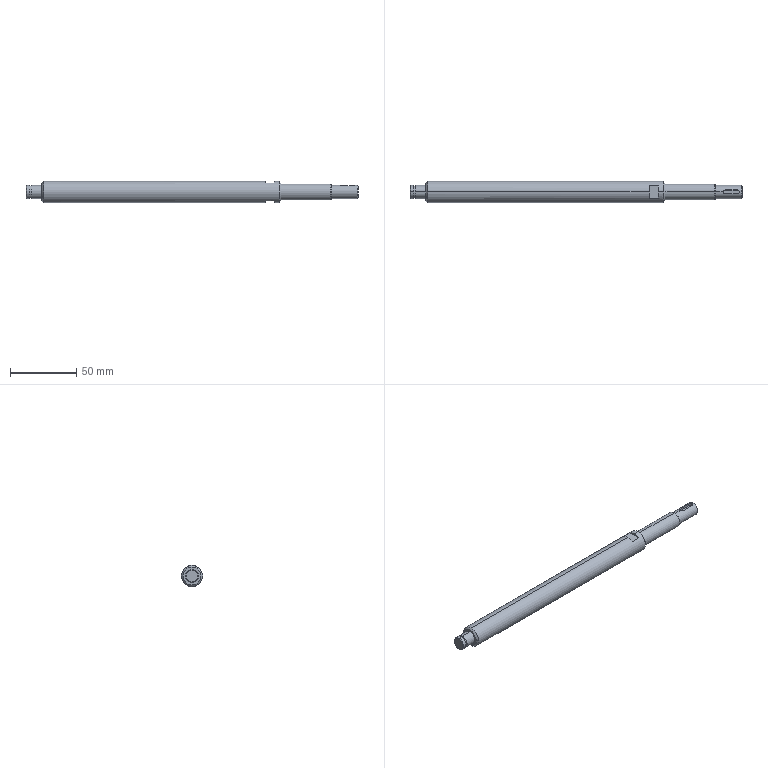Part | SolidWorks | features BaseBody 1 | 1 solid | 41 faces | box 250 x 16 x 16 mm | volume 42719 mm3 | plane 16 | cylinder 15 | cone 10 | commonest cylinder face diameters 10 x6 3 x3 9.6 x2 12 x2 16 x2
STEP:
#1=CARTESIAN_POINT('',(190.773,8.,0.));
#2=VERTEX_POINT('',#1);
#3=CARTESIAN_POINT('',(190.773,0.,-8.));
#4=VERTEX_POINT('',#3);
#5=CARTESIAN_POINT('',(190.773,0.,0.));
#6=DIRECTION('',(-1.,0.,0.));
#7=DIRECTION('',(0.,0.,1.));
#8=AXIS2_PLACEMENT_3D('',#5,#6,#7);
#9=CIRCLE('',#8,8.);
#10=EDGE_CURVE('',#2,#4,#9,.T.);
#11=ORIENTED_EDGE('',*,*,#10,.T.);
#12=CARTESIAN_POINT('',(187.,0.,-8.));
#13=VERTEX_POINT('',#12);
#14=CARTESIAN_POINT('',(250.,0.,-8.));
#15=DIRECTION('',(-1.,0.,0.));
#16=VECTOR('',#15,1000.);
#17=LINE('',#14,#16);
#18=EDGE_CURVE('',#4,#13,#17,.T.);
#19=ORIENTED_EDGE('',*,*,#18,.T.);
#20=CARTESIAN_POINT('',(187.,4.664,-6.5));
#21=VERTEX_POINT('',#20);
#22=CARTESIAN_POINT('',(187.,0.,0.));
#23=DIRECTION('',(1.,0.,0.));
#24=DIRECTION('',(0.,0.,1.));
#25=AXIS2_PLACEMENT_3D('',#22,#23,#24);
#26=CIRCLE('',#25,8.);
#27=EDGE_CURVE('',#13,#21,#26,.T.);
#28=ORIENTED_EDGE('',*,*,#27,.T.);
#29=CARTESIAN_POINT('',(180.,4.664,-6.5));
#30=VERTEX_POINT('',#29);
#31=CARTESIAN_POINT('',(250.,4.664,-6.5));
#32=DIRECTION('',(-1.,0.,0.));
#33=VECTOR('',#32,1000.);
#34=LINE('',#31,#33);
#35=EDGE_CURVE('',#21,#30,#34,.T.);
#36=ORIENTED_EDGE('',*,*,#35,.T.);
#37=CARTESIAN_POINT('',(180.,0.,-8.));
#38=VERTEX_POINT('',#37);
#39=CARTESIAN_POINT('',(180.,0.,0.));
#40=DIRECTION('',(-1.,0.,0.));
#41=DIRECTION('',(0.,0.,1.));
#42=AXIS2_PLACEMENT_3D('',#39,#40,#41);
#43=CIRCLE('',#42,8.);
#44=EDGE_CURVE('',#30,#38,#43,.T.);
#45=ORIENTED_EDGE('',*,*,#44,.T.);
#46=CARTESIAN_POINT('',(13.227,0.,-8.));
#47=VERTEX_POINT('',#46);
#48=CARTESIAN_POINT('',(250.,0.,-8.));
#49=DIRECTION('',(-1.,0.,0.));
#50=VECTOR('',#49,1000.);
#51=LINE('',#48,#50);
#52=EDGE_CURVE('',#38,#47,#51,.T.);
#53=ORIENTED_EDGE('',*,*,#52,.T.);
#54=CARTESIAN_POINT('',(13.227,8.,0.));
#55=VERTEX_POINT('',#54);
#56=CARTESIAN_POINT('',(13.227,0.,0.));
#57=DIRECTION('',(1.,0.,0.));
#58=DIRECTION('',(0.,0.,1.));
#59=AXIS2_PLACEMENT_3D('',#56,#57,#58);
#60=CIRCLE('',#59,8.);
#61=EDGE_CURVE('',#47,#55,#60,.T.);
#62=ORIENTED_EDGE('',*,*,#61,.T.);
#63=CARTESIAN_POINT('',(13.227,0.,8.));
#64=VERTEX_POINT('',#63);
#65=CARTESIAN_POINT('',(13.227,0.,0.));
#66=DIRECTION('',(1.,0.,0.));
#67=DIRECTION('',(0.,0.,1.));
#68=AXIS2_PLACEMENT_3D('',#65,#66,#67);
#69=CIRCLE('',#68,8.);
#70=EDGE_CURVE('',#55,#64,#69,.T.);
#71=ORIENTED_EDGE('',*,*,#70,.T.);
#72=CARTESIAN_POINT('',(180.,0.,8.));
#73=VERTEX_POINT('',#72);
#74=CARTESIAN_POINT('',(250.,0.,8.));
#75=DIRECTION('',(-1.,0.,0.));
#76=VECTOR('',#75,1000.);
#77=LINE('',#74,#76);
#78=EDGE_CURVE('',#73,#64,#77,.T.);
#79=ORIENTED_EDGE('',*,*,#78,.F.);
#80=CARTESIAN_POINT('',(180.,4.664,6.5));
#81=VERTEX_POINT('',#80);
#82=CARTESIAN_POINT('',(180.,0.,0.));
#83=DIRECTION('',(-1.,0.,0.));
#84=DIRECTION('',(0.,0.,1.));
#85=AXIS2_PLACEMENT_3D('',#82,#83,#84);
#86=CIRCLE('',#85,8.);
#87=EDGE_CURVE('',#73,#81,#86,.T.);
#88=ORIENTED_EDGE('',*,*,#87,.T.);
#89=CARTESIAN_POINT('',(187.,4.664,6.5));
#90=VERTEX_POINT('',#89);
#91=CARTESIAN_POINT('',(250.,4.664,6.5));
#92=DIRECTION('',(1.,0.,0.));
#93=VECTOR('',#92,1000.);
#94=LINE('',#91,#93);
#95=EDGE_CURVE('',#81,#90,#94,.T.);
#96=ORIENTED_EDGE('',*,*,#95,.T.);
#97=CARTESIAN_POINT('',(187.,0.,8.));
#98=VERTEX_POINT('',#97);
#99=CARTESIAN_POINT('',(187.,0.,0.));
#100=DIRECTION('',(1.,0.,0.));
#101=DIRECTION('',(0.,0.,1.));
#102=AXIS2_PLACEMENT_3D('',#99,#100,#101);
#103=CIRCLE('',#102,8.);
#104=EDGE_CURVE('',#90,#98,#103,.T.);
#105=ORIENTED_EDGE('',*,*,#104,.T.);
#106=CARTESIAN_POINT('',(190.773,0.,8.));
#107=VERTEX_POINT('',#106);
#108=CARTESIAN_POINT('',(250.,0.,8.));
#109=DIRECTION('',(-1.,0.,0.));
#110=VECTOR('',#109,1000.);
#111=LINE('',#108,#110);
#112=EDGE_CURVE('',#107,#98,#111,.T.);
#113=ORIENTED_EDGE('',*,*,#112,.F.);
#114=CARTESIAN_POINT('',(190.773,0.,0.));
#115=DIRECTION('',(-1.,0.,0.));
#116=DIRECTION('',(0.,0.,1.));
#117=AXIS2_PLACEMENT_3D('',#114,#115,#116);
#118=CIRCLE('',#117,8.);
#119=EDGE_CURVE('',#107,#2,#118,.T.);
#120=ORIENTED_EDGE('',*,*,#119,.T.);
#121=EDGE_LOOP('',(#11,#19,#28,#36,#45,#53,#62,#71,#79,#88,#96,#105,#113,#120));
#122=FACE_OUTER_BOUND('',#121,.T.);
#123=CARTESIAN_POINT('',(250.,0.,0.));
#124=DIRECTION('',(-1.,0.,0.));
#125=DIRECTION('',(0.,0.,1.));
#126=AXIS2_PLACEMENT_3D('',#123,#124,#125);
#127=CYLINDRICAL_SURFACE('',#126,8.);
#128=ADVANCED_FACE('',(#122),#127,.T.);
#129=CARTESIAN_POINT('',(12.,6.773,0.));
#130=VERTEX_POINT('',#129);
#131=CARTESIAN_POINT('',(12.,-6.773,0.));
#132=VERTEX_POINT('',#131);
#133=CARTESIAN_POINT('',(12.,0.,0.));
#134=DIRECTION('',(1.,0.,0.));
#135=DIRECTION('',(0.,1.,0.));
#136=AXIS2_PLACEMENT_3D('',#133,#134,#135);
#137=CIRCLE('',#136,6.773);
#138=EDGE_CURVE('',#130,#132,#137,.T.);
#139=ORIENTED_EDGE('',*,*,#138,.T.);
#140=CARTESIAN_POINT('',(13.227,-8.,0.));
#141=VERTEX_POINT('',#140);
#142=CARTESIAN_POINT('',(13.227,-8.,0.));
#143=DIRECTION('',(0.7071,-0.7071,0.));
#144=VECTOR('',#143,1000.);
#145=LINE('',#142,#144);
#146=EDGE_CURVE('',#132,#141,#145,.T.);
#147=ORIENTED_EDGE('',*,*,#146,.T.);
#148=CARTESIAN_POINT('',(13.227,0.,0.));
#149=DIRECTION('',(1.,0.,0.));
#150=DIRECTION('',(0.,0.,1.));
#151=AXIS2_PLACEMENT_3D('',#148,#149,#150);
#152=CIRCLE('',#151,8.);
#153=EDGE_CURVE('',#64,#141,#152,.T.);
#154=ORIENTED_EDGE('',*,*,#153,.F.);
#155=ORIENTED_EDGE('',*,*,#70,.F.);
#156=CARTESIAN_POINT('',(13.227,8.,0.));
#157=DIRECTION('',(0.7071,0.7071,0.));
#158=VECTOR('',#157,1000.);
#159=LINE('',#156,#158);
#160=EDGE_CURVE('',#130,#55,#159,.T.);
#161=ORIENTED_EDGE('',*,*,#160,.F.);
#162=EDGE_LOOP('',(#139,#147,#154,#155,#161));
#163=FACE_OUTER_BOUND('',#162,.T.);
#164=CARTESIAN_POINT('',(13.227,0.,0.));
#165=DIRECTION('',(1.,0.,0.));
#166=DIRECTION('',(0.,1.,0.));
#167=AXIS2_PLACEMENT_3D('',#164,#165,#166);
#168=CONICAL_SURFACE('',#167,8.,0.7854);
#169=ADVANCED_FACE('',(#163),#168,.T.);
#170=CARTESIAN_POINT('',(192.,-6.773,0.));
#171=VERTEX_POINT('',#170);
#172=CARTESIAN_POINT('',(192.,6.773,0.));
#173=VERTEX_POINT('',#172);
#174=CARTESIAN_POINT('',(192.,0.,0.));
#175=DIRECTION('',(-1.,0.,0.));
#176=DIRECTION('',(0.,-1.,0.));
#177=AXIS2_PLACEMENT_3D('',#174,#175,#176);
#178=CIRCLE('',#177,6.773);
#179=EDGE_CURVE('',#171,#173,#178,.T.);
#180=ORIENTED_EDGE('',*,*,#179,.T.);
#181=CARTESIAN_POINT('',(190.773,8.,0.));
#182=DIRECTION('',(-0.7071,0.7071,0.));
#183=VECTOR('',#182,1000.);
#184=LINE('',#181,#183);
#185=EDGE_CURVE('',#173,#2,#184,.T.);
#186=ORIENTED_EDGE('',*,*,#185,.T.);
#187=ORIENTED_EDGE('',*,*,#119,.F.);
#188=CARTESIAN_POINT('',(190.773,-8.,0.));
#189=VERTEX_POINT('',#188);
#190=CARTESIAN_POINT('',(190.773,0.,0.));
#191=DIRECTION('',(-1.,0.,0.));
#192=DIRECTION('',(0.,0.,1.));
#193=AXIS2_PLACEMENT_3D('',#190,#191,#192);
#194=CIRCLE('',#193,8.);
#195=EDGE_CURVE('',#189,#107,#194,.T.);
#196=ORIENTED_EDGE('',*,*,#195,.F.);
#197=CARTESIAN_POINT('',(190.773,-8.,0.));
#198=DIRECTION('',(-0.7071,-0.7071,0.));
#199=VECTOR('',#198,1000.);
#200=LINE('',#197,#199);
#201=EDGE_CURVE('',#171,#189,#200,.T.);
#202=ORIENTED_EDGE('',*,*,#201,.F.);
#203=EDGE_LOOP('',(#180,#186,#187,#196,#202));
#204=FACE_OUTER_BOUND('',#203,.T.);
#205=CARTESIAN_POINT('',(190.773,0.,0.));
#206=DIRECTION('',(-1.,0.,0.));
#207=DIRECTION('',(0.,-1.,0.));
#208=AXIS2_PLACEMENT_3D('',#205,#206,#207);
#209=CONICAL_SURFACE('',#208,8.,0.7854);
#210=ADVANCED_FACE('',(#204),#209,.T.);
#211=CARTESIAN_POINT('',(12.,0.,5.));
#212=VERTEX_POINT('',#211);
#213=CARTESIAN_POINT('',(12.,0.,-5.));
#214=VERTEX_POINT('',#213);
#215=CARTESIAN_POINT('',(12.,0.,0.));
#216=DIRECTION('',(-1.,0.,0.));
#217=DIRECTION('',(0.,0.,1.));
#218=AXIS2_PLACEMENT_3D('',#215,#216,#217);
#219=CIRCLE('',#218,5.);
#220=EDGE_CURVE('',#212,#214,#219,.T.);
#221=ORIENTED_EDGE('',*,*,#220,.T.);
#222=CARTESIAN_POINT('',(4.,0.,-5.));
#223=VERTEX_POINT('',#222);
#224=CARTESIAN_POINT('',(250.,0.,-5.));
#225=DIRECTION('',(-1.,0.,0.));
#226=VECTOR('',#225,1000.);
#227=LINE('',#224,#226);
#228=EDGE_CURVE('',#214,#223,#227,.T.);
#229=ORIENTED_EDGE('',*,*,#228,.T.);
#230=CARTESIAN_POINT('',(4.,0.,5.));
#231=VERTEX_POINT('',#230);
#232=CARTESIAN_POINT('',(4.,0.,0.));
#233=DIRECTION('',(1.,0.,0.));
#234=DIRECTION('',(0.,0.,1.));
#235=AXIS2_PLACEMENT_3D('',#232,#233,#234);
#236=CIRCLE('',#235,5.);
#237=EDGE_CURVE('',#223,#231,#236,.T.);
#238=ORIENTED_EDGE('',*,*,#237,.T.);
#239=CARTESIAN_POINT('',(250.,0.,5.));
#240=DIRECTION('',(-1.,0.,0.));
#241=VECTOR('',#240,1000.);
#242=LINE('',#239,#241);
#243=EDGE_CURVE('',#212,#231,#242,.T.);
#244=ORIENTED_EDGE('',*,*,#243,.F.);
#245=EDGE_LOOP('',(#221,#229,#238,#244));
#246=FACE_OUTER_BOUND('',#245,.T.);
#247=CARTESIAN_POINT('',(250.,0.,0.));
#248=DIRECTION('',(-1.,0.,0.));
#249=DIRECTION('',(0.,0.,1.));
#250=AXIS2_PLACEMENT_3D('',#247,#248,#249);
#251=CYLINDRICAL_SURFACE('',#250,5.);
#252=ADVANCED_FACE('',(#246),#251,.T.);
#253=CARTESIAN_POINT('',(229.5,0.,6.));
#254=VERTEX_POINT('',#253);
#255=CARTESIAN_POINT('',(229.5,0.,-6.));
#256=VERTEX_POINT('',#255);
#257=CARTESIAN_POINT('',(229.5,0.,0.));
#258=DIRECTION('',(-1.,0.,0.));
#259=DIRECTION('',(0.,0.,1.));
#260=AXIS2_PLACEMENT_3D('',#257,#258,#259);
#261=CIRCLE('',#260,6.);
#262=EDGE_CURVE('',#254,#256,#261,.T.);
#263=ORIENTED_EDGE('',*,*,#262,.T.);
#264=CARTESIAN_POINT('',(192.,0.,-6.));
#265=VERTEX_POINT('',#264);
#266=CARTESIAN_POINT('',(250.,0.,-6.));
#267=DIRECTION('',(-1.,0.,0.));
#268=VECTOR('',#267,1000.);
#269=LINE('',#266,#268);
#270=EDGE_CURVE('',#256,#265,#269,.T.);
#271=ORIENTED_EDGE('',*,*,#270,.T.);
#272=CARTESIAN_POINT('',(192.,0.,6.));
#273=VERTEX_POINT('',#272);
#274=CARTESIAN_POINT('',(192.,0.,0.));
#275=DIRECTION('',(1.,0.,0.));
#276=DIRECTION('',(0.,0.,1.));
#277=AXIS2_PLACEMENT_3D('',#274,#275,#276);
#278=CIRCLE('',#277,6.);
#279=EDGE_CURVE('',#265,#273,#278,.T.);
#280=ORIENTED_EDGE('',*,*,#279,.T.);
#281=CARTESIAN_POINT('',(250.,0.,6.));
#282=DIRECTION('',(-1.,0.,0.));
#283=VECTOR('',#282,1000.);
#284=LINE('',#281,#283);
#285=EDGE_CURVE('',#254,#273,#284,.T.);
#286=ORIENTED_EDGE('',*,*,#285,.F.);
#287=EDGE_LOOP('',(#263,#271,#280,#286));
#288=FACE_OUTER_BOUND('',#287,.T.);
#289=CARTESIAN_POINT('',(250.,0.,0.));
#290=DIRECTION('',(-1.,0.,0.));
#291=DIRECTION('',(0.,0.,1.));
#292=AXIS2_PLACEMENT_3D('',#289,#290,#291);
#293=CYLINDRICAL_SURFACE('',#292,6.);
#294=ADVANCED_FACE('',(#288),#293,.T.);
#295=CARTESIAN_POINT('',(230.,0.,5.5));
#296=VERTEX_POINT('',#295);
#297=CARTESIAN_POINT('',(230.,0.,-5.5));
#298=VERTEX_POINT('',#297);
#299=CARTESIAN_POINT('',(230.,0.,0.));
#300=DIRECTION('',(-1.,0.,0.));
#301=DIRECTION('',(0.,0.,1.));
#302=AXIS2_PLACEMENT_3D('',#299,#300,#301);
#303=CIRCLE('',#302,5.5);
#304=EDGE_CURVE('',#296,#298,#303,.T.);
#305=ORIENTED_EDGE('',*,*,#304,.T.);
#306=CARTESIAN_POINT('',(229.5,0.,-6.));
#307=DIRECTION('',(-0.7071,0.,-0.7071));
#308=VECTOR('',#307,1000.);
#309=LINE('',#306,#308);
#310=EDGE_CURVE('',#298,#256,#309,.T.);
#311=ORIENTED_EDGE('',*,*,#310,.T.);
#312=ORIENTED_EDGE('',*,*,#262,.F.);
#313=CARTESIAN_POINT('',(229.5,0.,6.));
#314=DIRECTION('',(-0.7071,0.,0.7071));
#315=VECTOR('',#314,1000.);
#316=LINE('',#313,#315);
#317=EDGE_CURVE('',#296,#254,#316,.T.);
#318=ORIENTED_EDGE('',*,*,#317,.F.);
#319=EDGE_LOOP('',(#305,#311,#312,#318));
#320=FACE_OUTER_BOUND('',#319,.T.);
#321=CARTESIAN_POINT('',(229.5,0.,0.));
#322=DIRECTION('',(-1.,0.,0.));
#323=DIRECTION('',(0.,0.,1.));
#324=AXIS2_PLACEMENT_3D('',#321,#322,#323);
#325=CONICAL_SURFACE('',#324,6.,0.7854);
#326=ADVANCED_FACE('',(#320),#325,.T.);
#327=CARTESIAN_POINT('',(4.,0.,4.8));
#328=VERTEX_POINT('',#327);
#329=CARTESIAN_POINT('',(4.,0.,-4.8));
#330=VERTEX_POINT('',#329);
#331=CARTESIAN_POINT('',(4.,0.,0.));
#332=DIRECTION('',(-1.,0.,0.));
#333=DIRECTION('',(0.,0.,1.));
#334=AXIS2_PLACEMENT_3D('',#331,#332,#333);
#335=CIRCLE('',#334,4.8);
#336=EDGE_CURVE('',#328,#330,#335,.T.);
#337=ORIENTED_EDGE('',*,*,#336,.T.);
#338=CARTESIAN_POINT('',(2.85,0.,-4.8));
#339=VERTEX_POINT('',#338);
#340=CARTESIAN_POINT('',(250.,0.,-4.8));
#341=DIRECTION('',(-1.,0.,0.));
#342=VECTOR('',#341,1000.);
#343=LINE('',#340,#342);
#344=EDGE_CURVE('',#330,#339,#343,.T.);
#345=ORIENTED_EDGE('',*,*,#344,.T.);
#346=CARTESIAN_POINT('',(2.85,0.,4.8));
#347=VERTEX_POINT('',#346);
#348=CARTESIAN_POINT('',(2.85,0.,0.));
#349=DIRECTION('',(1.,0.,0.));
#350=DIRECTION('',(0.,0.,1.));
#351=AXIS2_PLACEMENT_3D('',#348,#349,#350);
#352=CIRCLE('',#351,4.8);
#353=EDGE_CURVE('',#339,#347,#352,.T.);
#354=ORIENTED_EDGE('',*,*,#353,.T.);
#355=CARTESIAN_POINT('',(250.,0.,4.8));
#356=DIRECTION('',(-1.,0.,0.));
#357=VECTOR('',#356,1000.);
#358=LINE('',#355,#357);
#359=EDGE_CURVE('',#328,#347,#358,.T.);
#360=ORIENTED_EDGE('',*,*,#359,.F.);
#361=EDGE_LOOP('',(#337,#345,#354,#360));
#362=FACE_OUTER_BOUND('',#361,.T.);
#363=CARTESIAN_POINT('',(250.,0.,0.));
#364=DIRECTION('',(-1.,0.,0.));
#365=DIRECTION('',(0.,0.,1.));
#366=AXIS2_PLACEMENT_3D('',#363,#364,#365);
#367=CYLINDRICAL_SURFACE('',#366,4.8);
#368=ADVANCED_FACE('',(#362),#367,.T.);
#369=CARTESIAN_POINT('',(249.5,0.,5.));
#370=VERTEX_POINT('',#369);
#371=CARTESIAN_POINT('',(249.5,0.,-5.));
#372=VERTEX_POINT('',#371);
#373=CARTESIAN_POINT('',(249.5,0.,0.));
#374=DIRECTION('',(-1.,0.,0.));
#375=DIRECTION('',(0.,0.,1.));
#376=AXIS2_PLACEMENT_3D('',#373,#374,#375);
#377=CIRCLE('',#376,5.);
#378=EDGE_CURVE('',#370,#372,#377,.T.);
#379=ORIENTED_EDGE('',*,*,#378,.T.);
#380=CARTESIAN_POINT('',(230.,0.,-5.));
#381=VERTEX_POINT('',#380);
#382=CARTESIAN_POINT('',(250.,0.,-5.));
#383=DIRECTION('',(-1.,0.,0.));
#384=VECTOR('',#383,1000.);
#385=LINE('',#382,#384);
#386=EDGE_CURVE('',#372,#381,#385,.T.);
#387=ORIENTED_EDGE('',*,*,#386,.T.);
#388=CARTESIAN_POINT('',(230.,0.,5.));
#389=VERTEX_POINT('',#388);
#390=CARTESIAN_POINT('',(230.,0.,0.));
#391=DIRECTION('',(1.,0.,0.));
#392=DIRECTION('',(0.,0.,1.));
#393=AXIS2_PLACEMENT_3D('',#390,#391,#392);
#394=CIRCLE('',#393,5.);
#395=EDGE_CURVE('',#381,#389,#394,.T.);
#396=ORIENTED_EDGE('',*,*,#395,.T.);
#397=CARTESIAN_POINT('',(236.,0.,5.));
#398=VERTEX_POINT('',#397);
#399=CARTESIAN_POINT('',(250.,0.,5.));
#400=DIRECTION('',(-1.,0.,0.));
#401=VECTOR('',#400,1000.);
#402=LINE('',#399,#401);
#403=EDGE_CURVE('',#398,#389,#402,.T.);
#404=ORIENTED_EDGE('',*,*,#403,.F.);
#405=CARTESIAN_POINT('',(237.5,1.5,4.77));
#406=VERTEX_POINT('',#405);
#407=CARTESIAN_POINT('',(236.,0.,5.));
#408=CARTESIAN_POINT('',(236.,0.0984,5.));
#409=CARTESIAN_POINT('',(236.01,0.1984,4.997));
#410=CARTESIAN_POINT('',(236.049,0.391,4.986));
#411=CARTESIAN_POINT('',(236.077,0.4848,4.977));
#412=CARTESIAN_POINT('',(236.191,0.7581,4.946));
#413=CARTESIAN_POINT('',(236.301,0.9225,4.916));
#414=CARTESIAN_POINT('',(236.509,1.13,4.871));
#415=CARTESIAN_POINT('',(236.584,1.192,4.856));
#416=CARTESIAN_POINT('',(236.746,1.3,4.828));
#417=CARTESIAN_POINT('',(236.833,1.347,4.815));
#418=CARTESIAN_POINT('',(237.104,1.46,4.783));
#419=CARTESIAN_POINT('',(237.301,1.5,4.77));
#420=CARTESIAN_POINT('',(237.5,1.5,4.77));
#421=B_SPLINE_CURVE_WITH_KNOTS('',3,(#407,#408,#409,#410,#411,#412,#413,#414,#415,#416,#417,#418,#419,#420),.UNSPECIFIED.,.F.,.F.,(4,2,2,2,2,2,4),(0.002359,0.002654,0.002948,0.003537,0.003832,0.004126,0.004715),.UNSPECIFIED.);
#422=EDGE_CURVE('',#398,#406,#421,.T.);
#423=ORIENTED_EDGE('',*,*,#422,.T.);
#424=CARTESIAN_POINT('',(246.5,1.5,4.77));
#425=VERTEX_POINT('',#424);
#426=CARTESIAN_POINT('',(250.,1.5,4.77));
#427=DIRECTION('',(1.,0.,0.));
#428=VECTOR('',#427,1000.);
#429=LINE('',#426,#428);
#430=EDGE_CURVE('',#406,#425,#429,.T.);
#431=ORIENTED_EDGE('',*,*,#430,.T.);
#432=CARTESIAN_POINT('',(248.,0.,5.));
#433=VERTEX_POINT('',#432);
#434=CARTESIAN_POINT('',(246.5,1.5,4.77));
#435=CARTESIAN_POINT('',(246.6,1.5,4.77));
#436=CARTESIAN_POINT('',(246.698,1.49,4.773));
#437=CARTESIAN_POINT('',(246.89,1.452,4.785));
#438=CARTESIAN_POINT('',(246.986,1.423,4.794));
#439=CARTESIAN_POINT('',(247.167,1.347,4.815));
#440=CARTESIAN_POINT('',(247.253,1.301,4.828));
#441=CARTESIAN_POINT('',(247.416,1.192,4.856));
#442=CARTESIAN_POINT('',(247.492,1.129,4.871));
#443=CARTESIAN_POINT('',(247.699,0.9226,4.916));
#444=CARTESIAN_POINT('',(247.81,0.7561,4.946));
#445=CARTESIAN_POINT('',(247.96,0.3953,4.988));
#446=CARTESIAN_POINT('',(248.,0.197,5.));
#447=CARTESIAN_POINT('',(248.,0.,5.));
#448=B_SPLINE_CURVE_WITH_KNOTS('',3,(#434,#435,#436,#437,#438,#439,#440,#441,#442,#443,#444,#445,#446,#447),.UNSPECIFIED.,.F.,.F.,(4,2,2,2,2,2,4),(0.,0.0002949,0.0005898,0.0008847,0.00118,0.001769,0.002359),.UNSPECIFIED.);
#449=EDGE_CURVE('',#425,#433,#448,.T.);
#450=ORIENTED_EDGE('',*,*,#449,.T.);
#451=CARTESIAN_POINT('',(250.,0.,5.));
#452=DIRECTION('',(-1.,0.,0.));
#453=VECTOR('',#452,1000.);
#454=LINE('',#451,#453);
#455=EDGE_CURVE('',#370,#433,#454,.T.);
#456=ORIENTED_EDGE('',*,*,#455,.F.);
#457=EDGE_LOOP('',(#379,#387,#396,#404,#423,#431,#450,#456));
#458=FACE_OUTER_BOUND('',#457,.T.);
#459=CARTESIAN_POINT('',(250.,0.,0.));
#460=DIRECTION('',(-1.,0.,0.));
#461=DIRECTION('',(0.,0.,1.));
#462=AXIS2_PLACEMENT_3D('',#459,#460,#461);
#463=CYLINDRICAL_SURFACE('',#462,5.);
#464=ADVANCED_FACE('',(#458),#463,.T.);
#465=CARTESIAN_POINT('',(2.85,0.,5.));
#466=VERTEX_POINT('',#465);
#467=CARTESIAN_POINT('',(2.85,0.,-5.));
#468=VERTEX_POINT('',#467);
#469=CARTESIAN_POINT('',(2.85,0.,0.));
#470=DIRECTION('',(-1.,0.,0.));
#471=DIRECTION('',(0.,0.,1.));
#472=AXIS2_PLACEMENT_3D('',#469,#470,#471);
#473=CIRCLE('',#472,5.);
#474=EDGE_CURVE('',#466,#468,#473,.T.);
#475=ORIENTED_EDGE('',*,*,#474,.T.);
#476=CARTESIAN_POINT('',(0.5,0.,-5.));
#477=VERTEX_POINT('',#476);
#478=CARTESIAN_POINT('',(250.,0.,-5.));
#479=DIRECTION('',(-1.,0.,0.));
#480=VECTOR('',#479,1000.);
#481=LINE('',#478,#480);
#482=EDGE_CURVE('',#468,#477,#481,.T.);
#483=ORIENTED_EDGE('',*,*,#482,.T.);
#484=CARTESIAN_POINT('',(0.5,0.,5.));
#485=VERTEX_POINT('',#484);
#486=CARTESIAN_POINT('',(0.5,0.,0.));
#487=DIRECTION('',(1.,0.,0.));
#488=DIRECTION('',(0.,0.,1.));
#489=AXIS2_PLACEMENT_3D('',#486,#487,#488);
#490=CIRCLE('',#489,5.);
#491=EDGE_CURVE('',#477,#485,#490,.T.);
#492=ORIENTED_EDGE('',*,*,#491,.T.);
#493=CARTESIAN_POINT('',(250.,0.,5.));
#494=DIRECTION('',(-1.,0.,0.));
#495=VECTOR('',#494,1000.);
#496=LINE('',#493,#495);
#497=EDGE_CURVE('',#466,#485,#496,.T.);
#498=ORIENTED_EDGE('',*,*,#497,.F.);
#499=EDGE_LOOP('',(#475,#483,#492,#498));
#500=FACE_OUTER_BOUND('',#499,.T.);
#501=CARTESIAN_POINT('',(250.,0.,0.));
#502=DIRECTION('',(-1.,0.,0.));
#503=DIRECTION('',(0.,0.,1.));
#504=AXIS2_PLACEMENT_3D('',#501,#502,#503);
#505=CYLINDRICAL_SURFACE('',#504,5.);
#506=ADVANCED_FACE('',(#500),#505,.T.);
#507=ORIENTED_EDGE('',*,*,#422,.F.);
#508=CARTESIAN_POINT('',(236.,0.,3.2));
#509=VERTEX_POINT('',#508);
#510=CARTESIAN_POINT('',(236.,0.,3.2));
#511=DIRECTION('',(0.,0.,-1.));
#512=VECTOR('',#511,1000.);
#513=LINE('',#510,#512);
#514=EDGE_CURVE('',#398,#509,#513,.T.);
#515=ORIENTED_EDGE('',*,*,#514,.T.);
#516=CARTESIAN_POINT('',(237.5,1.5,3.2));
#517=VERTEX_POINT('',#516);
#518=CARTESIAN_POINT('',(237.5,0.,3.2));
#519=DIRECTION('',(0.,0.,1.));
#520=DIRECTION('',(-1.,0.,0.));
#521=AXIS2_PLACEMENT_3D('',#518,#519,#520);
#522=CIRCLE('',#521,1.5);
#523=EDGE_CURVE('',#517,#509,#522,.T.);
#524=ORIENTED_EDGE('',*,*,#523,.F.);
#525=CARTESIAN_POINT('',(237.5,1.5,3.2));
#526=DIRECTION('',(0.,0.,1.));
#527=VECTOR('',#526,1000.);
#528=LINE('',#525,#527);
#529=EDGE_CURVE('',#517,#406,#528,.T.);
#530=ORIENTED_EDGE('',*,*,#529,.T.);
#531=EDGE_LOOP('',(#507,#515,#524,#530));
#532=FACE_OUTER_BOUND('',#531,.T.);
#533=CARTESIAN_POINT('',(237.5,0.,3.2));
#534=DIRECTION('',(0.,0.,-1.));
#535=DIRECTION('',(-1.,0.,0.));
#536=AXIS2_PLACEMENT_3D('',#533,#534,#535);
#537=CYLINDRICAL_SURFACE('',#536,1.5);
#538=ADVANCED_FACE('',(#532),#537,.F.);
#539=CARTESIAN_POINT('',(250.,0.,4.5));
#540=VERTEX_POINT('',#539);
#541=CARTESIAN_POINT('',(250.,0.,-4.5));
#542=VERTEX_POINT('',#541);
#543=CARTESIAN_POINT('',(250.,0.,0.));
#544=DIRECTION('',(-1.,0.,0.));
#545=DIRECTION('',(0.,0.,1.));
#546=AXIS2_PLACEMENT_3D('',#543,#544,#545);
#547=CIRCLE('',#546,4.5);
#548=EDGE_CURVE('',#540,#542,#547,.T.);
#549=ORIENTED_EDGE('',*,*,#548,.T.);
#550=CARTESIAN_POINT('',(249.5,0.,-5.));
#551=DIRECTION('',(-0.7071,0.,-0.7071));
#552=VECTOR('',#551,1000.);
#553=LINE('',#550,#552);
#554=EDGE_CURVE('',#542,#372,#553,.T.);
#555=ORIENTED_EDGE('',*,*,#554,.T.);
#556=ORIENTED_EDGE('',*,*,#378,.F.);
#557=CARTESIAN_POINT('',(249.5,0.,5.));
#558=DIRECTION('',(-0.7071,0.,0.7071));
#559=VECTOR('',#558,1000.);
#560=LINE('',#557,#559);
#561=EDGE_CURVE('',#540,#370,#560,.T.);
#562=ORIENTED_EDGE('',*,*,#561,.F.);
#563=EDGE_LOOP('',(#549,#555,#556,#562));
#564=FACE_OUTER_BOUND('',#563,.T.);
#565=CARTESIAN_POINT('',(249.5,0.,0.));
#566=DIRECTION('',(-1.,0.,0.));
#567=DIRECTION('',(0.,0.,1.));
#568=AXIS2_PLACEMENT_3D('',#565,#566,#567);
#569=CONICAL_SURFACE('',#568,5.,0.7854);
#570=ADVANCED_FACE('',(#564),#569,.T.);
#571=CARTESIAN_POINT('',(0.,0.,-4.5));
#572=VERTEX_POINT('',#571);
#573=CARTESIAN_POINT('',(0.,0.,4.5));
#574=VERTEX_POINT('',#573);
#575=CARTESIAN_POINT('',(0.,0.,0.));
#576=DIRECTION('',(1.,0.,0.));
#577=DIRECTION('',(0.,0.,-1.));
#578=AXIS2_PLACEMENT_3D('',#575,#576,#577);
#579=CIRCLE('',#578,4.5);
#580=EDGE_CURVE('',#572,#574,#579,.T.);
#581=ORIENTED_EDGE('',*,*,#580,.T.);
#582=CARTESIAN_POINT('',(0.5,0.,5.));
#583=DIRECTION('',(0.7071,0.,0.7071));
#584=VECTOR('',#583,1000.);
#585=LINE('',#582,#584);
#586=EDGE_CURVE('',#574,#485,#585,.T.);
#587=ORIENTED_EDGE('',*,*,#586,.T.);
#588=ORIENTED_EDGE('',*,*,#491,.F.);
#589=CARTESIAN_POINT('',(0.5,0.,-5.));
#590=DIRECTION('',(0.7071,0.,-0.7071));
#591=VECTOR('',#590,1000.);
#592=LINE('',#589,#591);
#593=EDGE_CURVE('',#572,#477,#592,.T.);
#594=ORIENTED_EDGE('',*,*,#593,.F.);
#595=EDGE_LOOP('',(#581,#587,#588,#594));
#596=FACE_OUTER_BOUND('',#595,.T.);
#597=CARTESIAN_POINT('',(0.5,0.,0.));
#598=DIRECTION('',(1.,0.,0.));
#599=DIRECTION('',(0.,0.,-1.));
#600=AXIS2_PLACEMENT_3D('',#597,#598,#599);
#601=CONICAL_SURFACE('',#600,5.,0.7854);
#602=ADVANCED_FACE('',(#596),#601,.T.);
#603=ORIENTED_EDGE('',*,*,#18,.F.);
#604=CARTESIAN_POINT('',(190.773,0.,0.));
#605=DIRECTION('',(-1.,0.,0.));
#606=DIRECTION('',(0.,0.,1.));
#607=AXIS2_PLACEMENT_3D('',#604,#605,#606);
#608=CIRCLE('',#607,8.);
#609=EDGE_CURVE('',#4,#189,#608,.T.);
#610=ORIENTED_EDGE('',*,*,#609,.T.);
#611=ORIENTED_EDGE('',*,*,#195,.T.);
#612=ORIENTED_EDGE('',*,*,#112,.T.);
#613=CARTESIAN_POINT('',(187.,-4.664,6.5));
#614=VERTEX_POINT('',#613);
#615=CARTESIAN_POINT('',(187.,0.,0.));
#616=DIRECTION('',(1.,0.,0.));
#617=DIRECTION('',(0.,0.,1.));
#618=AXIS2_PLACEMENT_3D('',#615,#616,#617);
#619=CIRCLE('',#618,8.);
#620=EDGE_CURVE('',#98,#614,#619,.T.);
#621=ORIENTED_EDGE('',*,*,#620,.T.);
#622=CARTESIAN_POINT('',(180.,-4.664,6.5));
#623=VERTEX_POINT('',#622);
#624=CARTESIAN_POINT('',(250.,-4.664,6.5));
#625=DIRECTION('',(-1.,0.,0.));
#626=VECTOR('',#625,1000.);
#627=LINE('',#624,#626);
#628=EDGE_CURVE('',#614,#623,#627,.T.);
#629=ORIENTED_EDGE('',*,*,#628,.T.);
#630=CARTESIAN_POINT('',(180.,0.,0.));
#631=DIRECTION('',(-1.,0.,0.));
#632=DIRECTION('',(0.,0.,1.));
#633=AXIS2_PLACEMENT_3D('',#630,#631,#632);
#634=CIRCLE('',#633,8.);
#635=EDGE_CURVE('',#623,#73,#634,.T.);
#636=ORIENTED_EDGE('',*,*,#635,.T.);
#637=ORIENTED_EDGE('',*,*,#78,.T.);
#638=ORIENTED_EDGE('',*,*,#153,.T.);
#639=CARTESIAN_POINT('',(13.227,0.,0.));
#640=DIRECTION('',(1.,0.,0.));
#641=DIRECTION('',(0.,0.,1.));
#642=AXIS2_PLACEMENT_3D('',#639,#640,#641);
#643=CIRCLE('',#642,8.);
#644=EDGE_CURVE('',#141,#47,#643,.T.);
#645=ORIENTED_EDGE('',*,*,#644,.T.);
#646=ORIENTED_EDGE('',*,*,#52,.F.);
#647=CARTESIAN_POINT('',(180.,-4.664,-6.5));
#648=VERTEX_POINT('',#647);
#649=CARTESIAN_POINT('',(180.,0.,0.));
#650=DIRECTION('',(-1.,0.,0.));
#651=DIRECTION('',(0.,0.,1.));
#652=AXIS2_PLACEMENT_3D('',#649,#650,#651);
#653=CIRCLE('',#652,8.);
#654=EDGE_CURVE('',#38,#648,#653,.T.);
#655=ORIENTED_EDGE('',*,*,#654,.T.);
#656=CARTESIAN_POINT('',(187.,-4.664,-6.5));
#657=VERTEX_POINT('',#656);
#658=CARTESIAN_POINT('',(250.,-4.664,-6.5));
#659=DIRECTION('',(1.,0.,0.));
#660=VECTOR('',#659,1000.);
#661=LINE('',#658,#660);
#662=EDGE_CURVE('',#648,#657,#661,.T.);
#663=ORIENTED_EDGE('',*,*,#662,.T.);
#664=CARTESIAN_POINT('',(187.,0.,0.));
#665=DIRECTION('',(1.,0.,0.));
#666=DIRECTION('',(0.,0.,1.));
#667=AXIS2_PLACEMENT_3D('',#664,#665,#666);
#668=CIRCLE('',#667,8.);
#669=EDGE_CURVE('',#657,#13,#668,.T.);
#670=ORIENTED_EDGE('',*,*,#669,.T.);
#671=EDGE_LOOP('',(#603,#610,#611,#612,#621,#629,#636,#637,#638,#645,#646,#655,#663,#670));
#672=FACE_OUTER_BOUND('',#671,.T.);
#673=CARTESIAN_POINT('',(250.,0.,0.));
#674=DIRECTION('',(-1.,0.,0.));
#675=DIRECTION('',(0.,0.,1.));
#676=AXIS2_PLACEMENT_3D('',#673,#674,#675);
#677=CYLINDRICAL_SURFACE('',#676,8.);
#678=ADVANCED_FACE('',(#672),#677,.T.);
#679=ORIENTED_EDGE('',*,*,#95,.F.);
#680=CARTESIAN_POINT('',(180.,8.,6.5));
#681=DIRECTION('',(0.,-1.,0.));
#682=VECTOR('',#681,1000.);
#683=LINE('',#680,#682);
#684=EDGE_CURVE('',#81,#623,#683,.T.);
#685=ORIENTED_EDGE('',*,*,#684,.T.);
#686=ORIENTED_EDGE('',*,*,#628,.F.);
#687=CARTESIAN_POINT('',(187.,8.,6.5));
#688=DIRECTION('',(0.,1.,0.));
#689=VECTOR('',#688,1000.);
#690=LINE('',#687,#689);
#691=EDGE_CURVE('',#614,#90,#690,.T.);
#692=ORIENTED_EDGE('',*,*,#691,.T.);
#693=EDGE_LOOP('',(#679,#685,#686,#692));
#694=FACE_OUTER_BOUND('',#693,.T.);
#695=CARTESIAN_POINT('',(180.,8.,6.5));
#696=DIRECTION('',(0.,0.,1.));
#697=DIRECTION('',(1.,0.,0.));
#698=AXIS2_PLACEMENT_3D('',#695,#696,#697);
#699=PLANE('',#698);
#700=ADVANCED_FACE('',(#694),#699,.T.);
#701=ORIENTED_EDGE('',*,*,#104,.F.);
#702=ORIENTED_EDGE('',*,*,#691,.F.);
#703=ORIENTED_EDGE('',*,*,#620,.F.);
#704=EDGE_LOOP('',(#701,#702,#703));
#705=FACE_OUTER_BOUND('',#704,.T.);
#706=CARTESIAN_POINT('',(187.,0.,0.));
#707=DIRECTION('',(1.,0.,0.));
#708=DIRECTION('',(0.,0.,-1.));
#709=AXIS2_PLACEMENT_3D('',#706,#707,#708);
#710=PLANE('',#709);
#711=ADVANCED_FACE('',(#705),#710,.F.);
#712=ORIENTED_EDGE('',*,*,#635,.F.);
#713=ORIENTED_EDGE('',*,*,#684,.F.);
#714=ORIENTED_EDGE('',*,*,#87,.F.);
#715=EDGE_LOOP('',(#712,#713,#714));
#716=FACE_OUTER_BOUND('',#715,.T.);
#717=CARTESIAN_POINT('',(180.,0.,0.));
#718=DIRECTION('',(1.,0.,0.));
#719=DIRECTION('',(0.,0.,-1.));
#720=AXIS2_PLACEMENT_3D('',#717,#718,#719);
#721=PLANE('',#720);
#722=ADVANCED_FACE('',(#716),#721,.T.);
#723=ORIENTED_EDGE('',*,*,#146,.F.);
#724=CARTESIAN_POINT('',(12.,0.,0.));
#725=DIRECTION('',(1.,0.,0.));
#726=DIRECTION('',(0.,1.,0.));
#727=AXIS2_PLACEMENT_3D('',#724,#725,#726);
#728=CIRCLE('',#727,6.773);
#729=EDGE_CURVE('',#132,#130,#728,.T.);
#730=ORIENTED_EDGE('',*,*,#729,.T.);
#731=ORIENTED_EDGE('',*,*,#160,.T.);
#732=ORIENTED_EDGE('',*,*,#61,.F.);
#733=ORIENTED_EDGE('',*,*,#644,.F.);
#734=EDGE_LOOP('',(#723,#730,#731,#732,#733));
#735=FACE_OUTER_BOUND('',#734,.T.);
#736=CARTESIAN_POINT('',(13.227,0.,0.));
#737=DIRECTION('',(1.,0.,0.));
#738=DIRECTION('',(0.,1.,0.));
#739=AXIS2_PLACEMENT_3D('',#736,#737,#738);
#740=CONICAL_SURFACE('',#739,8.,0.7854);
#741=ADVANCED_FACE('',(#735),#740,.T.);
#742=ORIENTED_EDGE('',*,*,#662,.F.);
#743=CARTESIAN_POINT('',(180.,-8.,-6.5));
#744=DIRECTION('',(0.,1.,0.));
#745=VECTOR('',#744,1000.);
#746=LINE('',#743,#745);
#747=EDGE_CURVE('',#648,#30,#746,.T.);
#748=ORIENTED_EDGE('',*,*,#747,.T.);
#749=ORIENTED_EDGE('',*,*,#35,.F.);
#750=CARTESIAN_POINT('',(187.,-8.,-6.5));
#751=DIRECTION('',(0.,-1.,0.));
#752=VECTOR('',#751,1000.);
#753=LINE('',#750,#752);
#754=EDGE_CURVE('',#21,#657,#753,.T.);
#755=ORIENTED_EDGE('',*,*,#754,.T.);
#756=EDGE_LOOP('',(#742,#748,#749,#755));
#757=FACE_OUTER_BOUND('',#756,.T.);
#758=CARTESIAN_POINT('',(180.,-8.,-6.5));
#759=DIRECTION('',(0.,0.,-1.));
#760=DIRECTION('',(-1.,0.,0.));
#761=AXIS2_PLACEMENT_3D('',#758,#759,#760);
#762=PLANE('',#761);
#763=ADVANCED_FACE('',(#757),#762,.T.);
#764=ORIENTED_EDGE('',*,*,#669,.F.);
#765=ORIENTED_EDGE('',*,*,#754,.F.);
#766=ORIENTED_EDGE('',*,*,#27,.F.);
#767=EDGE_LOOP('',(#764,#765,#766));
#768=FACE_OUTER_BOUND('',#767,.T.);
#769=CARTESIAN_POINT('',(187.,0.,0.));
#770=DIRECTION('',(1.,0.,0.));
#771=DIRECTION('',(0.,0.,-1.));
#772=AXIS2_PLACEMENT_3D('',#769,#770,#771);
#773=PLANE('',#772);
#774=ADVANCED_FACE('',(#768),#773,.F.);
#775=ORIENTED_EDGE('',*,*,#44,.F.);
#776=ORIENTED_EDGE('',*,*,#747,.F.);
#777=ORIENTED_EDGE('',*,*,#654,.F.);
#778=EDGE_LOOP('',(#775,#776,#777));
#779=FACE_OUTER_BOUND('',#778,.T.);
#780=CARTESIAN_POINT('',(180.,0.,0.));
#781=DIRECTION('',(1.,0.,0.));
#782=DIRECTION('',(0.,0.,-1.));
#783=AXIS2_PLACEMENT_3D('',#780,#781,#782);
#784=PLANE('',#783);
#785=ADVANCED_FACE('',(#779),#784,.T.);
#786=ORIENTED_EDGE('',*,*,#185,.F.);
#787=CARTESIAN_POINT('',(192.,0.,0.));
#788=DIRECTION('',(-1.,0.,0.));
#789=DIRECTION('',(0.,-1.,0.));
#790=AXIS2_PLACEMENT_3D('',#787,#788,#789);
#791=CIRCLE('',#790,6.773);
#792=EDGE_CURVE('',#173,#171,#791,.T.);
#793=ORIENTED_EDGE('',*,*,#792,.T.);
#794=ORIENTED_EDGE('',*,*,#201,.T.);
#795=ORIENTED_EDGE('',*,*,#609,.F.);
#796=ORIENTED_EDGE('',*,*,#10,.F.);
#797=EDGE_LOOP('',(#786,#793,#794,#795,#796));
#798=FACE_OUTER_BOUND('',#797,.T.);
#799=CARTESIAN_POINT('',(190.773,0.,0.));
#800=DIRECTION('',(-1.,0.,0.));
#801=DIRECTION('',(0.,-1.,0.));
#802=AXIS2_PLACEMENT_3D('',#799,#800,#801);
#803=CONICAL_SURFACE('',#802,8.,0.7854);
#804=ADVANCED_FACE('',(#798),#803,.T.);
#805=ORIENTED_EDGE('',*,*,#220,.F.);
#806=CARTESIAN_POINT('',(12.,0.,0.));
#807=DIRECTION('',(-1.,0.,0.));
#808=DIRECTION('',(0.,0.,1.));
#809=AXIS2_PLACEMENT_3D('',#806,#807,#808);
#810=CIRCLE('',#809,5.);
#811=EDGE_CURVE('',#214,#212,#810,.T.);
#812=ORIENTED_EDGE('',*,*,#811,.F.);
#813=EDGE_LOOP('',(#805,#812));
#814=FACE_BOUND('',#813,.T.);
#815=ORIENTED_EDGE('',*,*,#138,.F.);
#816=ORIENTED_EDGE('',*,*,#729,.F.);
#817=EDGE_LOOP('',(#815,#816));
#818=FACE_OUTER_BOUND('',#817,.T.);
#819=CARTESIAN_POINT('',(12.,5.,0.));
#820=DIRECTION('',(1.,0.,0.));
#821=DIRECTION('',(0.,0.,-1.));
#822=AXIS2_PLACEMENT_3D('',#819,#820,#821);
#823=PLANE('',#822);
#824=ADVANCED_FACE('',(#814,#818),#823,.F.);
#825=ORIENTED_EDGE('',*,*,#179,.F.);
#826=ORIENTED_EDGE('',*,*,#792,.F.);
#827=EDGE_LOOP('',(#825,#826));
#828=FACE_OUTER_BOUND('',#827,.T.);
#829=CARTESIAN_POINT('',(192.,0.,0.));
#830=DIRECTION('',(1.,0.,0.));
#831=DIRECTION('',(0.,0.,1.));
#832=AXIS2_PLACEMENT_3D('',#829,#830,#831);
#833=CIRCLE('',#832,6.);
#834=EDGE_CURVE('',#273,#265,#833,.T.);
#835=ORIENTED_EDGE('',*,*,#834,.F.);
#836=ORIENTED_EDGE('',*,*,#279,.F.);
#837=EDGE_LOOP('',(#835,#836));
#838=FACE_BOUND('',#837,.T.);
#839=CARTESIAN_POINT('',(192.,6.773,0.));
#840=DIRECTION('',(-1.,0.,0.));
#841=DIRECTION('',(0.,0.,1.));
#842=AXIS2_PLACEMENT_3D('',#839,#840,#841);
#843=PLANE('',#842);
#844=ADVANCED_FACE('',(#828,#838),#843,.F.);
#845=ORIENTED_EDGE('',*,*,#228,.F.);
#846=ORIENTED_EDGE('',*,*,#811,.T.);
#847=ORIENTED_EDGE('',*,*,#243,.T.);
#848=CARTESIAN_POINT('',(4.,0.,0.));
#849=DIRECTION('',(1.,0.,0.));
#850=DIRECTION('',(0.,0.,1.));
#851=AXIS2_PLACEMENT_3D('',#848,#849,#850);
#852=CIRCLE('',#851,5.);
#853=EDGE_CURVE('',#231,#223,#852,.T.);
#854=ORIENTED_EDGE('',*,*,#853,.T.);
#855=EDGE_LOOP('',(#845,#846,#847,#854));
#856=FACE_OUTER_BOUND('',#855,.T.);
#857=CARTESIAN_POINT('',(250.,0.,0.));
#858=DIRECTION('',(-1.,0.,0.));
#859=DIRECTION('',(0.,0.,1.));
#860=AXIS2_PLACEMENT_3D('',#857,#858,#859);
#861=CYLINDRICAL_SURFACE('',#860,5.);
#862=ADVANCED_FACE('',(#856),#861,.T.);
#863=ORIENTED_EDGE('',*,*,#270,.F.);
#864=CARTESIAN_POINT('',(229.5,0.,0.));
#865=DIRECTION('',(-1.,0.,0.));
#866=DIRECTION('',(0.,0.,1.));
#867=AXIS2_PLACEMENT_3D('',#864,#865,#866);
#868=CIRCLE('',#867,6.);
#869=EDGE_CURVE('',#256,#254,#868,.T.);
#870=ORIENTED_EDGE('',*,*,#869,.T.);
#871=ORIENTED_EDGE('',*,*,#285,.T.);
#872=ORIENTED_EDGE('',*,*,#834,.T.);
#873=EDGE_LOOP('',(#863,#870,#871,#872));
#874=FACE_OUTER_BOUND('',#873,.T.);
#875=CARTESIAN_POINT('',(250.,0.,0.));
#876=DIRECTION('',(-1.,0.,0.));
#877=DIRECTION('',(0.,0.,1.));
#878=AXIS2_PLACEMENT_3D('',#875,#876,#877);
#879=CYLINDRICAL_SURFACE('',#878,6.);
#880=ADVANCED_FACE('',(#874),#879,.T.);
#881=ORIENTED_EDGE('',*,*,#336,.F.);
#882=CARTESIAN_POINT('',(4.,0.,0.));
#883=DIRECTION('',(-1.,0.,0.));
#884=DIRECTION('',(0.,0.,1.));
#885=AXIS2_PLACEMENT_3D('',#882,#883,#884);
#886=CIRCLE('',#885,4.8);
#887=EDGE_CURVE('',#330,#328,#886,.T.);
#888=ORIENTED_EDGE('',*,*,#887,.F.);
#889=EDGE_LOOP('',(#881,#888));
#890=FACE_BOUND('',#889,.T.);
#891=ORIENTED_EDGE('',*,*,#853,.F.);
#892=ORIENTED_EDGE('',*,*,#237,.F.);
#893=EDGE_LOOP('',(#891,#892));
#894=FACE_OUTER_BOUND('',#893,.T.);
#895=CARTESIAN_POINT('',(4.,4.8,0.));
#896=DIRECTION('',(1.,0.,0.));
#897=DIRECTION('',(0.,0.,-1.));
#898=AXIS2_PLACEMENT_3D('',#895,#896,#897);
#899=PLANE('',#898);
#900=ADVANCED_FACE('',(#890,#894),#899,.F.);
#901=ORIENTED_EDGE('',*,*,#310,.F.);
#902=CARTESIAN_POINT('',(230.,0.,0.));
#903=DIRECTION('',(-1.,0.,0.));
#904=DIRECTION('',(0.,0.,1.));
#905=AXIS2_PLACEMENT_3D('',#902,#903,#904);
#906=CIRCLE('',#905,5.5);
#907=EDGE_CURVE('',#298,#296,#906,.T.);
#908=ORIENTED_EDGE('',*,*,#907,.T.);
#909=ORIENTED_EDGE('',*,*,#317,.T.);
#910=ORIENTED_EDGE('',*,*,#869,.F.);
#911=EDGE_LOOP('',(#901,#908,#909,#910));
#912=FACE_OUTER_BOUND('',#911,.T.);
#913=CARTESIAN_POINT('',(229.5,0.,0.));
#914=DIRECTION('',(-1.,0.,0.));
#915=DIRECTION('',(0.,0.,1.));
#916=AXIS2_PLACEMENT_3D('',#913,#914,#915);
#917=CONICAL_SURFACE('',#916,6.,0.7854);
#918=ADVANCED_FACE('',(#912),#917,.T.);
#919=ORIENTED_EDGE('',*,*,#344,.F.);
#920=ORIENTED_EDGE('',*,*,#887,.T.);
#921=ORIENTED_EDGE('',*,*,#359,.T.);
#922=CARTESIAN_POINT('',(2.85,0.,0.));
#923=DIRECTION('',(1.,0.,0.));
#924=DIRECTION('',(0.,0.,1.));
#925=AXIS2_PLACEMENT_3D('',#922,#923,#924);
#926=CIRCLE('',#925,4.8);
#927=EDGE_CURVE('',#347,#339,#926,.T.);
#928=ORIENTED_EDGE('',*,*,#927,.T.);
#929=EDGE_LOOP('',(#919,#920,#921,#928));
#930=FACE_OUTER_BOUND('',#929,.T.);
#931=CARTESIAN_POINT('',(250.,0.,0.));
#932=DIRECTION('',(-1.,0.,0.));
#933=DIRECTION('',(0.,0.,1.));
#934=AXIS2_PLACEMENT_3D('',#931,#932,#933);
#935=CYLINDRICAL_SURFACE('',#934,4.8);
#936=ADVANCED_FACE('',(#930),#935,.T.);
#937=ORIENTED_EDGE('',*,*,#304,.F.);
#938=ORIENTED_EDGE('',*,*,#907,.F.);
#939=EDGE_LOOP('',(#937,#938));
#940=FACE_OUTER_BOUND('',#939,.T.);
#941=CARTESIAN_POINT('',(230.,0.,0.));
#942=DIRECTION('',(1.,0.,0.));
#943=DIRECTION('',(0.,0.,1.));
#944=AXIS2_PLACEMENT_3D('',#941,#942,#943);
#945=CIRCLE('',#944,5.);
#946=EDGE_CURVE('',#389,#381,#945,.T.);
#947=ORIENTED_EDGE('',*,*,#946,.F.);
#948=ORIENTED_EDGE('',*,*,#395,.F.);
#949=EDGE_LOOP('',(#947,#948));
#950=FACE_BOUND('',#949,.T.);
#951=CARTESIAN_POINT('',(230.,5.5,0.));
#952=DIRECTION('',(-1.,0.,0.));
#953=DIRECTION('',(0.,0.,1.));
#954=AXIS2_PLACEMENT_3D('',#951,#952,#953);
#955=PLANE('',#954);
#956=ADVANCED_FACE('',(#940,#950),#955,.F.);
#957=ORIENTED_EDGE('',*,*,#474,.F.);
#958=CARTESIAN_POINT('',(2.85,0.,0.));
#959=DIRECTION('',(-1.,0.,0.));
#960=DIRECTION('',(0.,0.,1.));
#961=AXIS2_PLACEMENT_3D('',#958,#959,#960);
#962=CIRCLE('',#961,5.);
#963=EDGE_CURVE('',#468,#466,#962,.T.);
#964=ORIENTED_EDGE('',*,*,#963,.F.);
#965=EDGE_LOOP('',(#957,#964));
#966=FACE_OUTER_BOUND('',#965,.T.);
#967=ORIENTED_EDGE('',*,*,#927,.F.);
#968=ORIENTED_EDGE('',*,*,#353,.F.);
#969=EDGE_LOOP('',(#967,#968));
#970=FACE_BOUND('',#969,.T.);
#971=CARTESIAN_POINT('',(2.85,5.,0.));
#972=DIRECTION('',(-1.,0.,0.));
#973=DIRECTION('',(0.,0.,1.));
#974=AXIS2_PLACEMENT_3D('',#971,#972,#973);
#975=PLANE('',#974);
#976=ADVANCED_FACE('',(#966,#970),#975,.F.);
#977=ORIENTED_EDGE('',*,*,#386,.F.);
#978=CARTESIAN_POINT('',(249.5,0.,0.));
#979=DIRECTION('',(-1.,0.,0.));
#980=DIRECTION('',(0.,0.,1.));
#981=AXIS2_PLACEMENT_3D('',#978,#979,#980);
#982=CIRCLE('',#981,5.);
#983=EDGE_CURVE('',#372,#370,#982,.T.);
#984=ORIENTED_EDGE('',*,*,#983,.T.);
#985=ORIENTED_EDGE('',*,*,#455,.T.);
#986=CARTESIAN_POINT('',(246.5,-1.5,4.77));
#987=VERTEX_POINT('',#986);
#988=CARTESIAN_POINT('',(248.,0.,5.));
#989=CARTESIAN_POINT('',(248.,-0.0984,5.));
#990=CARTESIAN_POINT('',(247.99,-0.1984,4.997));
#991=CARTESIAN_POINT('',(247.951,-0.391,4.986));
#992=CARTESIAN_POINT('',(247.923,-0.4848,4.977));
#993=CARTESIAN_POINT('',(247.809,-0.7581,4.946));
#994=CARTESIAN_POINT('',(247.699,-0.9225,4.916));
#995=CARTESIAN_POINT('',(247.491,-1.13,4.871));
#996=CARTESIAN_POINT('',(247.416,-1.192,4.856));
#997=CARTESIAN_POINT('',(247.254,-1.3,4.828));
#998=CARTESIAN_POINT('',(247.167,-1.347,4.815));
#999=CARTESIAN_POINT('',(246.896,-1.46,4.783));
#1000=CARTESIAN_POINT('',(246.699,-1.5,4.77));
#1001=CARTESIAN_POINT('',(246.5,-1.5,4.77));
#1002=B_SPLINE_CURVE_WITH_KNOTS('',3,(#988,#989,#990,#991,#992,#993,#994,#995,#996,#997,#998,#999,#1000,#1001),.UNSPECIFIED.,.F.,.F.,(4,2,2,2,2,2,4),(0.002359,0.002654,0.002948,0.003537,0.003832,0.004126,0.004715),.UNSPECIFIED.);
#1003=EDGE_CURVE('',#433,#987,#1002,.T.);
#1004=ORIENTED_EDGE('',*,*,#1003,.T.);
#1005=CARTESIAN_POINT('',(237.5,-1.5,4.77));
#1006=VERTEX_POINT('',#1005);
#1007=CARTESIAN_POINT('',(250.,-1.5,4.77));
#1008=DIRECTION('',(-1.,0.,0.));
#1009=VECTOR('',#1008,1000.);
#1010=LINE('',#1007,#1009);
#1011=EDGE_CURVE('',#987,#1006,#1010,.T.);
#1012=ORIENTED_EDGE('',*,*,#1011,.T.);
#1013=CARTESIAN_POINT('',(237.5,-1.5,4.77));
#1014=CARTESIAN_POINT('',(237.4,-1.5,4.77));
#1015=CARTESIAN_POINT('',(237.302,-1.49,4.773));
#1016=CARTESIAN_POINT('',(237.11,-1.452,4.785));
#1017=CARTESIAN_POINT('',(237.014,-1.423,4.794));
#1018=CARTESIAN_POINT('',(236.833,-1.347,4.815));
#1019=CARTESIAN_POINT('',(236.747,-1.301,4.828));
#1020=CARTESIAN_POINT('',(236.584,-1.192,4.856));
#1021=CARTESIAN_POINT('',(236.508,-1.129,4.871));
#1022=CARTESIAN_POINT('',(236.301,-0.9226,4.916));
#1023=CARTESIAN_POINT('',(236.19,-0.7561,4.946));
#1024=CARTESIAN_POINT('',(236.04,-0.3953,4.988));
#1025=CARTESIAN_POINT('',(236.,-0.197,5.));
#1026=CARTESIAN_POINT('',(236.,0.,5.));
#1027=B_SPLINE_CURVE_WITH_KNOTS('',3,(#1013,#1014,#1015,#1016,#1017,#1018,#1019,#1020,#1021,#1022,#1023,#1024,#1025,#1026),.UNSPECIFIED.,.F.,.F.,(4,2,2,2,2,2,4),(0.,0.0002949,0.0005898,0.0008847,0.00118,0.001769,0.002359),.UNSPECIFIED.);
#1028=EDGE_CURVE('',#1006,#398,#1027,.T.);
#1029=ORIENTED_EDGE('',*,*,#1028,.T.);
#1030=ORIENTED_EDGE('',*,*,#403,.T.);
#1031=ORIENTED_EDGE('',*,*,#946,.T.);
#1032=EDGE_LOOP('',(#977,#984,#985,#1004,#1012,#1029,#1030,#1031));
#1033=FACE_OUTER_BOUND('',#1032,.T.);
#1034=CARTESIAN_POINT('',(250.,0.,0.));
#1035=DIRECTION('',(-1.,0.,0.));
#1036=DIRECTION('',(0.,0.,1.));
#1037=AXIS2_PLACEMENT_3D('',#1034,#1035,#1036);
#1038=CYLINDRICAL_SURFACE('',#1037,5.);
#1039=ADVANCED_FACE('',(#1033),#1038,.T.);
#1040=ORIENTED_EDGE('',*,*,#482,.F.);
#1041=ORIENTED_EDGE('',*,*,#963,.T.);
#1042=ORIENTED_EDGE('',*,*,#497,.T.);
#1043=CARTESIAN_POINT('',(0.5,0.,0.));
#1044=DIRECTION('',(1.,0.,0.));
#1045=DIRECTION('',(0.,0.,1.));
#1046=AXIS2_PLACEMENT_3D('',#1043,#1044,#1045);
#1047=CIRCLE('',#1046,5.);
#1048=EDGE_CURVE('',#485,#477,#1047,.T.);
#1049=ORIENTED_EDGE('',*,*,#1048,.T.);
#1050=EDGE_LOOP('',(#1040,#1041,#1042,#1049));
#1051=FACE_OUTER_BOUND('',#1050,.T.);
#1052=CARTESIAN_POINT('',(250.,0.,0.));
#1053=DIRECTION('',(-1.,0.,0.));
#1054=DIRECTION('',(0.,0.,1.));
#1055=AXIS2_PLACEMENT_3D('',#1052,#1053,#1054);
#1056=CYLINDRICAL_SURFACE('',#1055,5.);
#1057=ADVANCED_FACE('',(#1051),#1056,.T.);
#1058=CARTESIAN_POINT('',(246.5,1.5,3.2));
#1059=VERTEX_POINT('',#1058);
#1060=CARTESIAN_POINT('',(246.5,1.5,3.2));
#1061=DIRECTION('',(-1.,0.,0.));
#1062=VECTOR('',#1061,1000.);
#1063=LINE('',#1060,#1062);
#1064=EDGE_CURVE('',#1059,#517,#1063,.T.);
#1065=ORIENTED_EDGE('',*,*,#1064,.F.);
#1066=CARTESIAN_POINT('',(246.5,1.5,3.2));
#1067=DIRECTION('',(0.,0.,-1.));
#1068=VECTOR('',#1067,1000.);
#1069=LINE('',#1066,#1068);
#1070=EDGE_CURVE('',#425,#1059,#1069,.T.);
#1071=ORIENTED_EDGE('',*,*,#1070,.F.);
#1072=ORIENTED_EDGE('',*,*,#430,.F.);
#1073=ORIENTED_EDGE('',*,*,#529,.F.);
#1074=EDGE_LOOP('',(#1065,#1071,#1072,#1073));
#1075=FACE_OUTER_BOUND('',#1074,.T.);
#1076=CARTESIAN_POINT('',(246.5,1.5,3.2));
#1077=DIRECTION('',(0.,1.,0.));
#1078=DIRECTION('',(0.,0.,1.));
#1079=AXIS2_PLACEMENT_3D('',#1076,#1077,#1078);
#1080=PLANE('',#1079);
#1081=ADVANCED_FACE('',(#1075),#1080,.F.);
#1082=ORIENTED_EDGE('',*,*,#514,.F.);
#1083=ORIENTED_EDGE('',*,*,#1028,.F.);
#1084=CARTESIAN_POINT('',(237.5,-1.5,3.2));
#1085=VERTEX_POINT('',#1084);
#1086=CARTESIAN_POINT('',(237.5,-1.5,3.2));
#1087=DIRECTION('',(0.,0.,1.));
#1088=VECTOR('',#1087,1000.);
#1089=LINE('',#1086,#1088);
#1090=EDGE_CURVE('',#1085,#1006,#1089,.T.);
#1091=ORIENTED_EDGE('',*,*,#1090,.F.);
#1092=CARTESIAN_POINT('',(237.5,0.,3.2));
#1093=DIRECTION('',(0.,0.,1.));
#1094=DIRECTION('',(-1.,0.,0.));
#1095=AXIS2_PLACEMENT_3D('',#1092,#1093,#1094);
#1096=CIRCLE('',#1095,1.5);
#1097=EDGE_CURVE('',#509,#1085,#1096,.T.);
#1098=ORIENTED_EDGE('',*,*,#1097,.F.);
#1099=EDGE_LOOP('',(#1082,#1083,#1091,#1098));
#1100=FACE_OUTER_BOUND('',#1099,.T.);
#1101=CARTESIAN_POINT('',(237.5,0.,3.2));
#1102=DIRECTION('',(0.,0.,-1.));
#1103=DIRECTION('',(-1.,0.,0.));
#1104=AXIS2_PLACEMENT_3D('',#1101,#1102,#1103);
#1105=CYLINDRICAL_SURFACE('',#1104,1.5);
#1106=ADVANCED_FACE('',(#1100),#1105,.F.);
#1107=CARTESIAN_POINT('',(246.5,-1.5,3.2));
#1108=VERTEX_POINT('',#1107);
#1109=CARTESIAN_POINT('',(237.5,-1.5,3.2));
#1110=DIRECTION('',(1.,0.,0.));
#1111=VECTOR('',#1110,1000.);
#1112=LINE('',#1109,#1111);
#1113=EDGE_CURVE('',#1085,#1108,#1112,.T.);
#1114=ORIENTED_EDGE('',*,*,#1113,.F.);
#1115=ORIENTED_EDGE('',*,*,#1090,.T.);
#1116=ORIENTED_EDGE('',*,*,#1011,.F.);
#1117=CARTESIAN_POINT('',(246.5,-1.5,3.2));
#1118=DIRECTION('',(0.,0.,1.));
#1119=VECTOR('',#1118,1000.);
#1120=LINE('',#1117,#1119);
#1121=EDGE_CURVE('',#1108,#987,#1120,.T.);
#1122=ORIENTED_EDGE('',*,*,#1121,.F.);
#1123=EDGE_LOOP('',(#1114,#1115,#1116,#1122));
#1124=FACE_OUTER_BOUND('',#1123,.T.);
#1125=CARTESIAN_POINT('',(237.5,-1.5,3.2));
#1126=DIRECTION('',(0.,-1.,0.));
#1127=DIRECTION('',(0.,0.,-1.));
#1128=AXIS2_PLACEMENT_3D('',#1125,#1126,#1127);
#1129=PLANE('',#1128);
#1130=ADVANCED_FACE('',(#1124),#1129,.F.);
#1131=ORIENTED_EDGE('',*,*,#449,.F.);
#1132=ORIENTED_EDGE('',*,*,#1070,.T.);
#1133=CARTESIAN_POINT('',(246.5,0.,3.2));
#1134=DIRECTION('',(0.,0.,1.));
#1135=DIRECTION('',(-1.,0.,0.));
#1136=AXIS2_PLACEMENT_3D('',#1133,#1134,#1135);
#1137=CIRCLE('',#1136,1.5);
#1138=EDGE_CURVE('',#1108,#1059,#1137,.T.);
#1139=ORIENTED_EDGE('',*,*,#1138,.F.);
#1140=ORIENTED_EDGE('',*,*,#1121,.T.);
#1141=ORIENTED_EDGE('',*,*,#1003,.F.);
#1142=EDGE_LOOP('',(#1131,#1132,#1139,#1140,#1141));
#1143=FACE_OUTER_BOUND('',#1142,.T.);
#1144=CARTESIAN_POINT('',(246.5,0.,3.2));
#1145=DIRECTION('',(0.,0.,-1.));
#1146=DIRECTION('',(-1.,0.,0.));
#1147=AXIS2_PLACEMENT_3D('',#1144,#1145,#1146);
#1148=CYLINDRICAL_SURFACE('',#1147,1.5);
#1149=ADVANCED_FACE('',(#1143),#1148,.F.);
#1150=ORIENTED_EDGE('',*,*,#554,.F.);
#1151=CARTESIAN_POINT('',(250.,0.,0.));
#1152=DIRECTION('',(-1.,0.,0.));
#1153=DIRECTION('',(0.,0.,1.));
#1154=AXIS2_PLACEMENT_3D('',#1151,#1152,#1153);
#1155=CIRCLE('',#1154,4.5);
#1156=EDGE_CURVE('',#542,#540,#1155,.T.);
#1157=ORIENTED_EDGE('',*,*,#1156,.T.);
#1158=ORIENTED_EDGE('',*,*,#561,.T.);
#1159=ORIENTED_EDGE('',*,*,#983,.F.);
#1160=EDGE_LOOP('',(#1150,#1157,#1158,#1159));
#1161=FACE_OUTER_BOUND('',#1160,.T.);
#1162=CARTESIAN_POINT('',(249.5,0.,0.));
#1163=DIRECTION('',(-1.,0.,0.));
#1164=DIRECTION('',(0.,0.,1.));
#1165=AXIS2_PLACEMENT_3D('',#1162,#1163,#1164);
#1166=CONICAL_SURFACE('',#1165,5.,0.7854);
#1167=ADVANCED_FACE('',(#1161),#1166,.T.);
#1168=ORIENTED_EDGE('',*,*,#586,.F.);
#1169=CARTESIAN_POINT('',(0.,0.,0.));
#1170=DIRECTION('',(1.,0.,0.));
#1171=DIRECTION('',(0.,0.,-1.));
#1172=AXIS2_PLACEMENT_3D('',#1169,#1170,#1171);
#1173=CIRCLE('',#1172,4.5);
#1174=EDGE_CURVE('',#574,#572,#1173,.T.);
#1175=ORIENTED_EDGE('',*,*,#1174,.T.);
#1176=ORIENTED_EDGE('',*,*,#593,.T.);
#1177=ORIENTED_EDGE('',*,*,#1048,.F.);
#1178=EDGE_LOOP('',(#1168,#1175,#1176,#1177));
#1179=FACE_OUTER_BOUND('',#1178,.T.);
#1180=CARTESIAN_POINT('',(0.5,0.,0.));
#1181=DIRECTION('',(1.,0.,0.));
#1182=DIRECTION('',(0.,0.,-1.));
#1183=AXIS2_PLACEMENT_3D('',#1180,#1181,#1182);
#1184=CONICAL_SURFACE('',#1183,5.,0.7854);
#1185=ADVANCED_FACE('',(#1179),#1184,.T.);
#1186=ORIENTED_EDGE('',*,*,#1138,.T.);
#1187=ORIENTED_EDGE('',*,*,#1064,.T.);
#1188=ORIENTED_EDGE('',*,*,#523,.T.);
#1189=ORIENTED_EDGE('',*,*,#1097,.T.);
#1190=ORIENTED_EDGE('',*,*,#1113,.T.);
#1191=EDGE_LOOP('',(#1186,#1187,#1188,#1189,#1190));
#1192=FACE_OUTER_BOUND('',#1191,.T.);
#1193=CARTESIAN_POINT('',(237.5,0.,3.2));
#1194=DIRECTION('',(0.,0.,1.));
#1195=DIRECTION('',(1.,0.,0.));
#1196=AXIS2_PLACEMENT_3D('',#1193,#1194,#1195);
#1197=PLANE('',#1196);
#1198=ADVANCED_FACE('',(#1192),#1197,.T.);
#1199=ORIENTED_EDGE('',*,*,#548,.F.);
#1200=ORIENTED_EDGE('',*,*,#1156,.F.);
#1201=EDGE_LOOP('',(#1199,#1200));
#1202=FACE_OUTER_BOUND('',#1201,.T.);
#1203=CARTESIAN_POINT('',(250.,4.5,0.));
#1204=DIRECTION('',(-1.,0.,0.));
#1205=DIRECTION('',(0.,0.,1.));
#1206=AXIS2_PLACEMENT_3D('',#1203,#1204,#1205);
#1207=PLANE('',#1206);
#1208=ADVANCED_FACE('',(#1202),#1207,.F.);
#1209=ORIENTED_EDGE('',*,*,#580,.F.);
#1210=ORIENTED_EDGE('',*,*,#1174,.F.);
#1211=EDGE_LOOP('',(#1209,#1210));
#1212=FACE_OUTER_BOUND('',#1211,.T.);
#1213=CARTESIAN_POINT('',(0.,0.,0.));
#1214=DIRECTION('',(1.,0.,0.));
#1215=DIRECTION('',(0.,0.,-1.));
#1216=AXIS2_PLACEMENT_3D('',#1213,#1214,#1215);
#1217=PLANE('',#1216);
#1218=ADVANCED_FACE('',(#1212),#1217,.F.);
#1219=CLOSED_SHELL('',(#128,#169,#210,#252,#294,#326,#368,#464,#506,#538,#570,#602,#678,#700,#711,#722,#741,#763,#774,#785,#804,#824,#844,#862,#880,#900,#918,#936,#956,#976,#1039,#1057,#1081,#1106,#1130,#1149,#1167,#1185,#1198,#1208,#1218));
#1220=MANIFOLD_SOLID_BREP('',#1219);
#1221=CARTESIAN_POINT('',(0.,0.,0.));
#1222=DIRECTION('',(0.,0.,1.));
#1223=DIRECTION('',(1.,0.,0.));
#1224=AXIS2_PLACEMENT_3D('',#1221,#1222,#1223);
#1225=(LENGTH_UNIT()NAMED_UNIT(*)SI_UNIT(.MILLI.,.METRE.));
#1226=UNCERTAINTY_MEASURE_WITH_UNIT(LENGTH_MEASURE(0.00001),#1225,'','');
#1227=(NAMED_UNIT(*)PLANE_ANGLE_UNIT()SI_UNIT($,.RADIAN.));
#1228=(NAMED_UNIT(*)SI_UNIT($,.STERADIAN.)SOLID_ANGLE_UNIT());
#1229=(GEOMETRIC_REPRESENTATION_CONTEXT(3)GLOBAL_UNCERTAINTY_ASSIGNED_CONTEXT((#1226))GLOBAL_UNIT_ASSIGNED_CONTEXT((#1225,#1227,#1228))REPRESENTATION_CONTEXT('',''));
#1230=ADVANCED_BREP_SHAPE_REPRESENTATION('',(#1220,#1224),#1229);